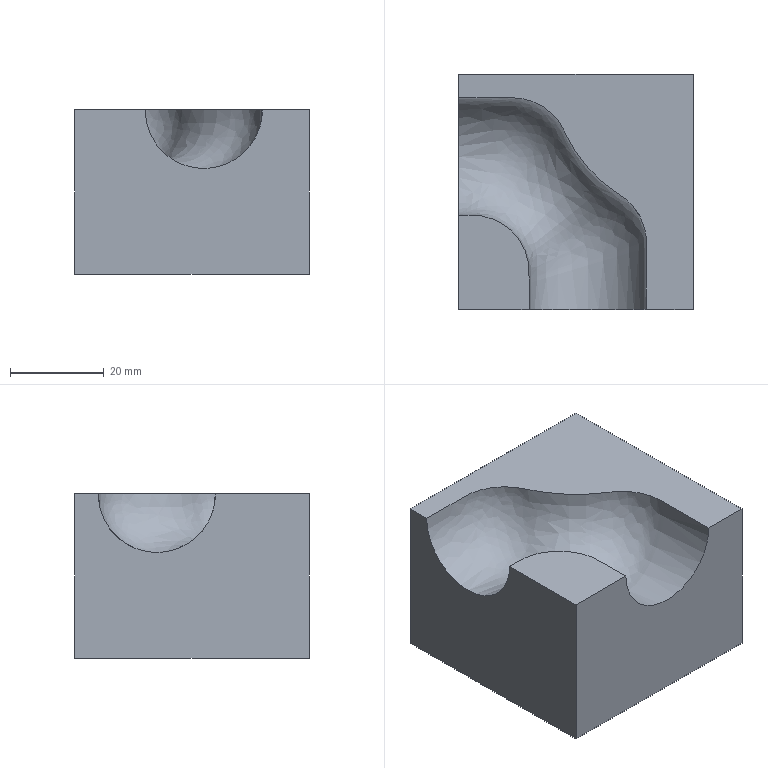NC program | NX | posted with a generic post | part box 50 x 50 x 35 mm
Lines 1308 to 2416 of 32931:
(CAVITY_MILL_COPY , TOOL : D6)
N2614 M6
N2616 G54
N2618 G17 G0 G90 X-3.401 Y23.101 S3000 M3
N2620 G43 Z10. H0
N2622 Z0.05
N2624 G94 G1 Z-0.15 F2500.
N2626 X0. Y23.1
N2628 X2.871 Y23.099
N2630 G2 X18.098 Y8.253 R15.092
N2632 G1 X18.102 Y0.
N2634 X18.103 Y-3.399
N2636 Z0.05
N2638 G0 Z0.3
N2640 X36.899
N2642 Z0.05
N2644 G1 Z-0.15
N2646 X36.898 Y0.
N2648 X36.896 Y14.233
N2650 G3 X32.772 Y21.732 R8.945
N2652 G2 X19.737 Y36.582 R33.162
N2654 G3 X11.611 Y41.89 R8.932
N2656 G1 X10.047 Y41.897
N2658 X0.479 Y41.896
N2660 X0. Y41.898
N2662 X-3.411 Y41.91
N2664 Z0.05
N2666 G0 Z0.3
N2668 X-3.404 Y23.103
N2670 Z-0.1
N2672 G1 Z-0.3
N2674 X0. Y23.104
N2676 X2.871
N2678 G2 X18.102 Y8.253 R15.093
N2680 G1 X18.106 Y0.
N2682 X18.108 Y-3.398
N2684 Z-0.1
N2686 G0 Z0.15
N2688 X36.894
N2690 Z-0.1
N2692 G1 Z-0.3
N2694 Y0.
N2696 X36.893 Y14.233
N2698 G3 X32.772 Y21.728 R8.987
N2700 G2 X19.732 Y36.58 R33.175
N2702 G3 X11.629 Y41.882 R8.925
N2704 G1 X10.047 Y41.891
N2706 X0.479 Y41.892
N2708 X0. Y41.894
N2710 X-3.413 Y41.906
N2712 Z-0.1
N2714 G0 Z0.15
N2716 X-3.408 Y23.105
N2718 Z-0.25
N2720 G1 Z-0.45
N2722 X0. Y23.108
N2724 X2.871 Y23.11
N2726 G2 X18.108 Y8.253 R15.1
N2728 G1 X18.111 Y0.
N2730 X18.113 Y-3.398
N2732 Z-0.25
N2734 G0 Z0.
N2736 X36.89 Y-3.4
N2738 Z-0.25
N2740 G1 Z-0.45
N2742 X36.889 Y0.
N2744 X36.888 Y14.233
N2746 G3 X32.772 Y21.72 R9.003
N2748 G2 X19.728 Y36.575 R33.21
N2750 G3 X11.589 Y41.872 R8.923
N2752 G1 X0. Y41.89
N2754 X-3.407 Y41.895
N2756 Z-0.25
N2758 G0 Z0.
N2760 X-3.414 Y23.106
N2762 Z-0.4
N2764 G1 Z-0.6
N2766 X0. Y23.113
N2768 X2.273 Y23.119
N2770 X2.871 Y23.118
N2772 G2 X11.91 Y20.213 R15.186
N2774 G1 X12.439 Y19.807
N2776 X12.677 Y19.615
N2778 X13.037 Y19.305
N2780 X13.386 Y19.017
N2782 G2 X17.883 Y10.645 R15.216
N2784 G1 X17.969 Y10.047
N2786 G2 X18.116 Y7.655 R16.334
N2788 G1 Y0.
N2790 Y-3.402
N2792 Z-0.4
N2794 G0 Z-0.15
N2796 X36.886 Y-3.405
N2798 Z-0.4
N2800 G1 Z-0.6
N2802 X36.885 Y0.
N2804 X36.883 Y14.233
N2806 G3 X32.772 Y21.713 R9.021
N2808 G2 X19.725 Y36.568 R33.239
N2810 G3 X11.607 Y41.864 R8.924
N2812 G1 X10.645 Y41.868
N2814 X0. Y41.879
N2816 X-3.4 Y41.882
N2818 Z-0.4
N2820 G0 Z-0.15
N2822 X-3.41 Y23.119
N2824 Z-0.55
N2826 G1 Z-0.75
N2828 X0. Y23.123
N2830 X2.871 Y23.125
N2832 G2 X11.841 Y20.272 R15.186
N2834 G1 X12.439 Y19.82
N2836 G2 X16.027 Y15.696 R14.321
N2838 X18.119 Y8.253 R15.038
N2840 G1 X18.124 Y0.
N2842 X18.126 Y-3.404
N2844 Z-0.55
N2846 G0 Z-0.3
N2848 X36.892 Y-3.42
N2850 Z-0.55
N2852 G1 Z-0.75
N2854 X36.875 Y0.
N2856 X36.873 Y0.479
N2858 X36.875 Y13.635
N2860 X36.871 Y14.233
N2862 G3 X32.772 Y21.699 R8.983
N2864 G2 X19.701 Y36.597 R33.251
N2866 G3 X11.648 Y41.855 R8.845
N2868 G1 X10.645 Y41.859
N2870 X0. Y41.867
N2872 X-3.398 Y41.87
N2874 Z-0.55
N2876 G0 Z-0.3
N2878 X-3.411 Y23.129
N2880 Z-0.7
N2882 G1 Z-0.9
N2884 X0. Y23.134
N2886 X2.871 Y23.138
N2888 X3.469 Y23.125
N2890 G2 X13.037 Y19.327 R15.12
N2892 G1 X13.42 Y19.017
N2894 G3 X14.233 Y18.183 R12.651
N2896 G1 X14.522 Y17.821
N2898 X14.831 Y17.439
N2900 X15.024 Y17.223
N2902 G2 X17.821 Y11.024 R15.031
N2904 G1 X17.903 Y10.645
N2906 X17.994 Y10.047
N2908 X18.066 Y9.449
N2910 X18.101 Y8.851
N2912 X18.131 Y8.253
N2914 X18.137 Y7.655
N2916 X18.144 Y0.479
N2918 X18.141 Y0.
N2920 X18.126 Y-3.415
N2922 Z-0.7
N2924 G0 Z-0.45
N2926 X36.877 Y-3.418
N2928 Z-0.7
N2930 G1 Z-0.9
N2932 X36.862 Y0.
N2934 X36.86 Y0.479
N2936 X36.863 Y13.635
N2938 X36.858 Y14.233
N2940 G3 X32.772 Y21.68 R8.913
N2942 G2 X21.689 Y32.772 R33.333
N2944 X19.726 Y36.529 R32.02
N2946 G3 X11.841 Y41.846 R8.916
N2948 G1 X0. Y41.856
N2950 X-3.398 Y41.859
N2952 Z-0.7
N2954 G0 Z-0.45
N2956 X-3.41 Y23.142
N2958 Z-0.85
N2960 G1 Z-1.05
N2962 X0. Y23.148
N2964 X2.871 Y23.154
N2966 X3.469 Y23.134
N2968 G2 X13.037 Y19.351 R15.19
N2970 G1 X13.437 Y19.017
N2972 X13.635 Y18.788
N2974 G2 X14.531 Y17.821 R7.059
N2976 X17.654 Y11.841 R14.809
N2978 X18.147 Y8.253 R15.68
N2980 G1 X18.153 Y7.655
N2982 X18.16 Y0.479
N2984 X18.158 Y0.
N2986 X18.144 Y-3.41
N2988 Z-0.85
N2990 G0 Z-0.6
N2992 X36.862 Y-3.417
N2994 Z-0.85
N2996 G1 Z-1.05
N2998 X36.848 Y0.
N3000 X36.846 Y0.479
N3002 X36.85 Y13.635
N3004 X36.846 Y14.233
N3006 G3 X33.37 Y21.256 R8.93
N3008 G1 X33.153 Y21.409
N3010 X32.257 Y22.007
N3012 X32.174 Y22.051
N3014 G2 X23.728 Y29.782 R32.398
N3016 X19.798 Y36.36 R32.22
N3018 G3 X17.757 Y39.35 R9.751
N3020 X11.841 Y41.837 R8.944
N3022 G1 X0. Y41.845
N3024 X-3.398 Y41.847
N3026 Z-0.85
N3028 G0 Z-0.6
N3030 X-3.411 Y23.156
N3032 Z-1.
N3034 G1 Z-1.2
N3036 X0. Y23.163
N3038 X2.871 Y23.169
N3040 X3.469 Y23.15
N3042 G2 X12.439 Y19.876 R15.361
N3044 X18.091 Y9.449 R15.063
N3046 G1 X18.163 Y8.253
N3048 X18.168 Y7.655
N3050 X18.175 Y0.
N3052 X18.177 Y-3.391
N3054 Z-1.
N3056 G0 Z-0.75
N3058 X36.847 Y-3.417
N3060 Z-1.
N3062 G1 Z-1.2
N3064 X36.835 Y0.
N3066 X36.833 Y0.479
N3068 X36.838 Y13.635
N3070 X36.834 Y14.271
N3072 G3 X33.321 Y21.261 R8.822
N3074 X32.174 Y22.034 R13.031
N3076 G2 X19.781 Y36.36 R32.749
N3078 G3 X17.746 Y39.35 R9.753
N3080 X11.841 Y41.829 R9.09
N3082 G1 X0. Y41.834
N3084 X-3.398 Y41.835
N3086 Z-1.
N3088 G0 Z-0.75
N3090 X-3.467 Y23.108
N3092 Z-1.15
N3094 G1 Z-1.35
N3096 X0. Y23.18
N3098 G2 X3.621 Y23.151 R62.449
N3100 X18.01 Y10.234 R15.109
N3102 X18.184 Y7.655 R16.706
N3104 G1 X18.192 Y0.008
N3106 Y0.
N3108 X18.187 Y-3.401
N3110 Z-1.15
N3112 G0 Z-0.9
N3114 X36.822 Y-3.407
N3116 Z-1.15
N3118 G1 Z-1.35
N3120 Y0.
N3122 X36.821 Y14.233
N3124 G3 X33.37 Y21.209 R8.848
N3126 G1 X33.095 Y21.409
N3128 X31.576 Y22.4
N3130 G2 X19.615 Y36.685 R32.788
N3132 G3 X13.635 Y41.577 R8.913
N3134 X11.841 Y41.82 R12.805
N3136 G1 X10.645 Y41.823
N3138 X0.479 Y41.821
N3140 X0. Y41.822
N3142 X-3.409 Y41.832
N3144 Z-1.15
N3146 G0 Z-0.9
N3148 X-3.415 Y23.184
N3150 Z-1.3
N3152 G1 Z-1.5
N3154 X0. Y23.193
N3156 X2.871 Y23.201
N3158 X3.469 Y23.183
N3160 G2 X17.347 Y13.037 R15.177
N3162 X18.195 Y8.253 R16.139
N3164 G1 X18.202 Y7.057
N3166 X18.209 Y0.007
N3168 Y0.
N3170 X18.205 Y-3.4
N3172 Z-1.3
N3174 G0 Z-1.05
N3176 X36.808 Y-3.41
N3178 Z-1.3
N3180 G1 Z-1.5
N3182 Y0.
N3184 X36.809 Y14.233
N3186 G3 X33.968 Y20.696 R8.958
N3188 X32.155 Y22.007 R14.236
N3190 G2 X19.743 Y36.36 R32.656
N3192 G3 X14.94 Y41.144 R8.948
N3194 X11.243 Y41.809 R9.702
N3196 G1 X0.479 Y41.804
N3198 X0. Y41.806
N3200 X-3.415 Y41.82
N3202 Z-1.3
N3204 G0 Z-1.05
N3206 X-3.422 Y23.197
N3208 Z-1.45
N3210 G1 Z-1.65
N3212 X0. Y23.211
N3214 X2.871 Y23.222
N3216 X3.469 Y23.199
N3218 G2 X17.369 Y13.037 R15.184
N3220 X18.212 Y7.93 R16.075
N3222 G1 X18.225 Y0.
N3224 X18.231 Y-3.39
N3226 Z-1.45
N3228 G0 Z-1.2
N3230 X36.784 Y-3.405
N3232 Z-1.45
N3234 G1 Z-1.65
N3236 Y0.
N3238 X36.788 Y14.233
N3240 G3 X33.37 Y21.161 R8.826
N3242 G1 X33.019 Y21.409
N3244 X31.208 Y22.605
N3246 G2 X19.721 Y36.36 R32.588
N3248 G3 X14.888 Y41.144 R8.922
N3250 X11.243 Y41.789 R9.65
N3252 G1 X0. Y41.786
N3254 X-3.403
N3256 Z-1.45
N3258 G0 Z-1.2
N3260 X-3.414 Y23.226
N3262 Z-1.6
N3264 G1 Z-1.8
N3266 X0. Y23.236
N3268 X2.871 Y23.245
N3270 X3.469 Y23.222
N3272 G2 X15.976 Y16.027 R15.288
N3274 X18.227 Y8.253 R15.352
N3276 G1 X18.231 Y7.655
N3278 X18.244 Y0.479
N3280 X18.243 Y0.
N3282 X18.237 Y-3.405
N3284 Z-1.6
N3286 G0 Z-1.35
N3288 X36.759 Y-3.4
N3290 Z-1.6
N3292 G1 Z-1.8
N3294 X36.76 Y0.
N3296 X36.766 Y14.233
N3298 G3 X32.772 Y21.561 R8.792
N3300 G2 X21.206 Y33.379 R32.856
N3302 X19.665 Y36.441 R31.796
N3304 G3 X11.841 Y41.767 R8.898
N3306 G1 X0. Y41.766
N3308 X-3.404
N3310 Z-1.6
N3312 G0 Z-1.35
N3314 X-3.405 Y23.254
N3316 Z-1.75
N3318 G1 Z-1.95
N3320 X0. Y23.262
N3322 X2.871 Y23.268
N3324 X3.469 Y23.247
N3326 G2 X14.233 Y18.363 R15.434
N3328 X18.243 Y8.253 R15.114
N3330 G1 X18.259 Y0.
N3332 X18.266 Y-3.399
N3334 Z-1.75
N3336 G0 Z-1.5
N3338 X36.734 Y-3.396
N3340 Z-1.75
N3342 G1 Z-1.95
N3344 X36.736 Y0.
N3346 X36.743 Y14.194
N3348 G3 X32.591 Y21.644 R8.751
N3350 G2 X26.792 Y26.126 R35.109
N3352 X19.641 Y36.444 R32.684
N3354 G3 X11.522 Y41.75 R8.859
N3356 G1 X0. Y41.745
N3358 X-3.406 Y41.744
N3360 Z-1.75
N3362 G0 Z-1.5
N3364 X-3.402 Y23.283
N3366 Z-1.9
N3368 G1 Z-2.1
N3370 X0. Y23.287
N3372 X2.871 Y23.291
N3374 X3.469 Y23.272
N3376 G2 X13.618 Y19.017 R15.495
N3378 X18.121 Y10.047 R14.77
N3380 X18.259 Y8.253 R12.285
N3382 G1 X18.281 Y0.
N3384 X18.29 Y-3.398
N3386 Z-1.9
N3388 G0 Z-1.65
N3390 X36.722 Y-3.407
N3392 Z-1.9
N3394 G1 Z-2.1
N3396 X36.712 Y0.
N3398 X36.71 Y0.479
N3400 X36.726 Y13.635
N3402 X36.721 Y14.233
N3404 G3 X32.772 Y21.504 R8.721
N3406 G2 X29.184 Y23.999 R38.773
N3408 X19.935 Y35.762 R32.106
N3410 G3 X19.262 Y37.142 R17.898
N3412 X11.562 Y41.724 R8.749
N3414 G1 X0. Y41.715
N3416 X-3.399 Y41.712
N3418 Z-1.9
N3420 G0 Z-1.65
N3422 X-3.401 Y23.312
N3424 Z-2.05
N3426 G1 Z-2.25
N3428 X0. Y23.313
N3430 X2.871 Y23.314
N3432 G2 X13.635 Y19.041 R15.623
N3434 X17.948 Y11.243 R14.636
N3436 X18.279 Y8.253 R14.6
N3438 G1 X18.311 Y0.
N3440 X18.324 Y-3.389
N3442 Z-2.05
N3444 G0 Z-1.8
N3446 X36.697 Y-3.408
N3448 Z-2.05
N3450 G1 Z-2.25
N3452 X36.687 Y0.
N3454 X36.686 Y0.479
N3456 X36.703 Y13.635
N3458 X36.699 Y14.233
N3460 G3 X32.772 Y21.474 R8.709
N3462 G2 X31.456 Y22.325 R116.378
N3464 X19.621 Y36.39 R32.097
N3466 G3 X11.535 Y41.692 R8.805
N3468 G1 X0. Y41.682
N3470 X-3.391 Y41.678
N3472 Z-2.05
N3474 G0 Z-1.8
N3476 X-3.404 Y23.341
N3478 Z-2.2
N3480 G1 Z-2.4
N3482 X0. Y23.338
N3484 X2.871 Y23.336
N3486 G2 X14.177 Y18.55 R15.647
N3488 X17.411 Y13.306 R14.466
N3490 X18.306 Y8.253 R15.847
N3492 G1 X18.341 Y0.005
N3494 Y0.
N3496 X18.349 Y-3.395
N3498 Z-2.2
N3500 G0 Z-1.95
N3502 X36.671 Y-3.41
N3504 Z-2.2
N3506 G1 Z-2.4
N3508 X36.663 Y0.
N3510 X36.662 Y0.479
N3512 X36.681 Y13.635
N3514 X36.677 Y14.233
N3516 G3 X32.772 Y21.445 R8.766
N3518 G2 X30.958 Y22.625 R53.384
N3520 X19.617 Y36.348 R31.874
N3522 G3 X11.528 Y41.661 R8.801
N3524 G1 X0.012 Y41.649
N3526 X0.
N3528 X-3.402 Y41.658
N3530 Z-2.2
N3532 G0 Z-1.95
N3534 X-3.39 Y23.39
N3536 Z-2.35
N3538 G1 Z-2.55
N3540 X0. Y23.367
N3542 X4.067 Y23.34
N3544 G2 X9.449 Y21.944 R16.364
N3546 X16.625 Y15.212 R15.269
N3548 X18.334 Y8.253 R15.742
N3550 G1 X18.371 Y0.007
N3552 Y0.
N3554 X18.379 Y-3.395
N3556 Z-2.35
N3558 G0 Z-2.1
N3560 X36.623 Y-3.393
N3562 Z-2.35
N3564 G1 Z-2.55
N3566 X36.629 Y0.
N3568 X36.652 Y14.233
N3570 G3 X33.968 Y20.455 R8.879
N3572 X32.174 Y21.802 R11.572
N3574 G1 X31.838 Y22.007
N3576 G2 X19.577 Y36.36 R31.869
N3578 G3 X11.841 Y41.625 R8.743
N3580 G1 X11.243 Y41.629
N3582 X0. Y41.615
N3584 X-3.374 Y41.611
N3586 Z-2.35
N3588 G0 Z-2.1
N3590 X-3.414 Y23.397
N3592 Z-2.5
N3594 G1 Z-2.7
N3596 X0. Y23.403
N3598 X0.479 Y23.404
N3600 X2.871 Y23.397
N3602 G2 X11.243 Y21.006 R15.591
N3604 G1 X11.559 Y20.811
N3606 G2 X17.585 Y13.037 R14.848
N3608 G1 X17.746 Y12.439
N3610 X17.821 Y12.176
N3612 X17.92 Y11.841
N3614 X18.085 Y11.001
N3616 G2 X18.362 Y8.213 R14.88
N3618 G1 X18.401 Y0.005
N3620 Y0.
N3622 X18.411 Y-3.394
N3624 Z-2.5
N3626 G0 Z-2.25
N3628 X36.595 Y-3.4
N3630 Z-2.5
N3632 G1 Z-2.7
N3634 X36.591 Y0.
N3636 Y0.009
N3638 X36.617 Y14.233
N3640 G3 X32.721 Y21.409 R8.731
N3642 G2 X30.287 Y23.01 R37.222
N3644 X19.546 Y36.349 R31.859
N3646 G3 X11.591 Y41.597 R8.672
N3648 X0. Y41.583 R2175.918
N3650 G1 X-3.382 Y41.569
N3652 Z-2.5
N3654 G0 Z-2.25
N3656 X-3.39 Y23.458
N3658 Z-2.65
N3660 G1 Z-2.85
N3662 X0. Y23.437
N3664 X3.469 Y23.416
N3666 X4.067 Y23.404
N3668 G2 X13.037 Y19.765 R16.14
N3670 X17.401 Y13.635 R14.643
N3672 X18.389 Y8.253 R15.767
N3674 G1 X18.437 Y0.479
N3676 X18.436 Y0.
N3678 X18.433 Y-3.401
N3680 Z-2.65
N3682 G0 Z-2.4
N3684 X36.56
N3686 Z-2.65
N3688 G1 Z-2.85
N3690 X36.553 Y0.
N3692 Y0.012
N3694 X36.581 Y14.145
N3696 G3 X32.453 Y21.535 R8.649
N3698 G2 X30.384 Y22.898 R38.101
N3700 X19.518 Y36.33 R31.759
N3702 G3 X11.588 Y41.566 R8.636
N3704 X0. Y41.55 R2397.27
N3706 G1 X-3.384 Y41.537
N3708 Z-2.65
N3710 G0 Z-2.4
N3712 X-3.432 Y23.445
N3714 Z-2.8
N3716 G1 Z-3.
N3718 X0. Y23.474
N3720 G2 X4.067 Y23.435 R114.595
N3722 X13.635 Y19.296 R16.118
N3724 X17.223 Y14.176 R14.563
N3726 X18.103 Y11.243 R13.453
N3728 X18.399 Y8.851 R12.147
N3730 G1 X18.417 Y8.253
N3732 X18.477 Y0.024
N3734 Y0.
N3736 X18.476 Y-3.399
N3738 Z-2.8
N3740 G0 Z-2.55
N3742 X36.525
N3744 Z-2.8
N3746 G1 Z-3.
N3748 X36.515 Y0.
N3750 X36.514 Y0.479
N3752 X36.545 Y14.141
N3754 G3 X32.378 Y21.54 R8.619
N3756 G2 X26.194 Y26.362 R32.949
N3758 X19.485 Y36.324 R32.257
N3760 G3 X11.563 Y41.535 R8.605
N3762 G1 X0. Y41.516
N3764 X-3.381 Y41.511
N3766 Z-2.8
N3768 G0 Z-2.55
N3770 X-3.412 Y23.504
N3772 Z-2.95
N3774 G1 Z-3.15
N3776 X0. Y23.509
N3778 X0.479 Y23.51
N3780 X2.871 Y23.501
N3782 G2 X15.429 Y17.399 R15.884
N3784 X18.419 Y9.019 R15.08
N3786 G1 X18.455 Y8.253
N3788 X18.518 Y0.03
N3790 X18.519 Y0.
N3792 X18.511 Y-3.401
N3794 Z-2.95
N3796 G0 Z-2.7
N3798 X36.487 Y-3.4
N3800 Z-2.95
N3802 G1 Z-3.15
N3804 X36.478 Y0.
N3806 X36.476 Y0.479
N3808 X36.509 Y14.17
N3810 G3 X32.348 Y21.52 R8.536
N3812 G2 X23.801 Y28.973 R31.85
N3814 X19.458 Y36.302 R33.633
N3816 G3 X11.528 Y41.504 R8.622
N3818 G1 X0. Y41.483
N3820 X-3.394 Y41.477
N3822 Z-2.95
N3824 G0 Z-2.7
N3826 X-3.388 Y23.565
N3828 Z-3.099
N3830 G1 Z-3.299
N3832 X0. Y23.554
N3834 X2.871 Y23.545
N3836 X3.469 Y23.527
N3838 G2 X15.429 Y17.481 R15.912
N3840 X18.473 Y8.851 R15.304
N3842 G1 X18.495 Y8.253
N3844 X18.561 Y0.479
N3846 Y0.008
N3848 Y0.
N3850 X18.551 Y-3.403
N3852 Z-3.099
N3854 G0 Z-2.85
N3856 X36.448 Y-3.402
N3858 Z-3.099
N3860 G1 Z-3.299
N3862 X36.44 Y0.
N3864 X36.439 Y0.479
N3866 X36.473 Y14.233
N3868 G3 X32.174 Y21.587 R8.587
N3870 G2 X19.615 Y35.882 R31.002
N3872 G1 X19.398 Y36.36
N3874 G3 X14.831 Y40.825 R8.68
N3876 X11.243 Y41.472 R9.147
N3878 G1 X0. Y41.45
N3880 X-3.399 Y41.444
N3882 Z-3.099
N3884 G0 Z-2.85
N3886 X-3.395 Y23.596
N3888 Z-3.249
N3890 G1 Z-3.449
N3892 X0. Y23.6
N3894 X0.479 Y23.601
N3896 X2.871 Y23.59
N3898 G2 X14.123 Y19.017 R16.236
N3900 X18.102 Y11.841 R14.382
N3902 X18.535 Y8.253 R17.344
N3904 G1 X18.603 Y0.479
N3906 Y0.006
N3908 Y0.
N3910 X18.596 Y-3.401
N3912 Z-3.249
N3914 G0 Z-2.999
N3916 X36.393 Y-3.389
N3918 Z-3.249
N3920 G1 Z-3.449
N3922 X36.403 Y0.
N3924 X36.444 Y14.097
N3926 G3 X32.219 Y21.513 R8.577
N3928 G2 X19.876 Y35.231 R30.645
N3930 G3 X19.017 Y37.047 R67.322
N3932 X11.243 Y41.439 R8.648
N3934 G1 X0. Y41.405
N3936 X-3.391 Y41.395
N3938 Z-3.249
N3940 G0 Z-2.999
N3942 X-3.395 Y23.642
N3944 Z-3.399
N3946 G1 Z-3.599
N3948 X0. Y23.645
N3950 X0.479 Y23.646
N3952 X2.871 Y23.635
N3954 G2 X12.827 Y20.213 R16.447
N3956 X18.273 Y11.243 R14.503
N3958 X18.574 Y8.253 R18.487
N3960 X18.644 Y0. R552.236
N3962 G1 X18.648 Y-3.39
N3964 Z-3.399
N3966 G0 Z-3.149
N3968 X36.356 Y-3.394
N3970 Z-3.399
N3972 G1 Z-3.599
N3974 X36.365 Y0.
N3976 X36.402 Y14.233
N3978 G3 X32.313 Y21.409 R8.54
N3980 G2 X19.593 Y35.762 R30.544
N3982 G1 X19.326 Y36.36
N3984 G3 X14.831 Y40.728 R8.668
N3986 X11.532 Y41.394 R8.382
N3988 G1 X0.01 Y41.357
N3990 X0.
N3992 X-3.399 Y41.358
N3994 Z-3.399
N3996 G0 Z-3.149
N3998 X-3.382 Y23.702
N4000 Z-3.549
N4002 G1 Z-3.749
N4004 X0. Y23.69
N4006 X2.871 Y23.68
N4008 G2 X12.907 Y20.213 R16.586
N4010 X18.311 Y11.273 R14.449
N4012 X18.605 Y8.117 R19.633
N4014 G1 X18.684 Y1.675
N4016 X18.686 Y0.
N4018 X18.69 Y-3.394
N4020 Z-3.549
N4022 G0 Z-3.299
N4024 X36.309 Y-3.396
N4026 Z-3.549
N4028 G1 Z-3.749
N4030 X36.315 Y0.
N4032 Y0.007
N4034 X36.372 Y14.061
N4036 G3 X32.147 Y21.459 R8.529
N4038 G2 X19.431 Y36.032 R30.345
N4040 G3 X11.444 Y41.347 R8.616
N4042 G1 X0.012 Y41.309
N4044 X0.
N4046 X-3.399 Y41.311
N4048 Z-3.549
N4050 G0 Z-3.299
N4052 X-3.366 Y23.761
N4054 Z-3.699
N4056 G1 Z-3.899
N4058 X0. Y23.735
N4060 X3.469 Y23.708
N4062 X4.067 Y23.684
N4064 G2 X13.737 Y19.615 R17.005
N4066 X18.245 Y11.841 R14.598
N4068 G1 X18.357 Y11.26
N4070 G2 X18.643 Y8.452 R15.877
N4072 G1 X18.728 Y1.675
N4074 X18.731 Y0.
N4076 X18.736 Y-3.395
N4078 Z-3.699
N4080 G0 Z-3.449
N4082 X36.248 Y-3.378
N4084 Z-3.699
N4086 G1 Z-3.899
N4088 X36.263 Y0.
N4090 X36.327 Y14.044
N4092 G3 X32.113 Y21.429 R8.509
N4094 G2 X26.519 Y25.596 R31.428
N4096 G3 X25.596 Y26.511 R11.013
N4098 G2 X22.858 Y29.782 R39.083
N4100 X19.321 Y36.14 R34.678
N4102 G3 X11.483 Y41.301 R8.487
N4104 G1 X0.012 Y41.261
N4106 X0.
N4108 X-3.399 Y41.263
N4110 Z-3.699
N4112 G0 Z-3.449
N4114 X-3.364 Y23.806
N4116 Z-3.849
N4118 G1 Z-4.049
N4120 X0. Y23.78
N4122 X3.469 Y23.753
N4124 X4.067 Y23.731
N4126 G2 X13.827 Y19.615 R17.115
N4128 X17.326 Y14.831 R15.134
N4130 X18.679 Y8.851 R16.835
N4132 G1 X18.693 Y8.253
N4134 X18.786 Y0.479
N4136 Y0.005
N4138 Y0.
N4140 X18.783 Y-3.4
N4142 Z-3.849
N4144 G0 Z-3.599
N4146 X36.195 Y-3.375
N4148 Z-3.849
N4150 G1 Z-4.049
N4152 X36.211 Y0.
N4154 X36.277 Y14.054
N4156 G3 X32.06 Y21.396 R8.431
N4158 G2 X27.12 Y24.998 R28.735
N4160 X26.194 Y25.863 R5.21
N4162 X24.727 Y27.39 R15.376
N4164 X20.914 Y32.772 R28.878
N4166 X19.251 Y36.187 R42.129
N4168 G3 X11.509 Y41.256 R8.401
N4170 G1 X0.009 Y41.213
N4172 X0.
N4174 X-3.397 Y41.21
N4176 Z-3.849
N4178 G0 Z-3.599
N4180 X-3.405 Y23.809
N4182 Z-3.999
N4184 G1 Z-4.199
N4186 X0. Y23.835
N4188 G2 X4.067 Y23.777 R94.103
N4190 X13.917 Y19.615 R17.183
N4192 G1 X14.413 Y19.125
N4194 G2 X18.419 Y11.421 R14.174
N4196 X18.721 Y8.851 R15.586
N4198 G1 X18.836 Y1.675
N4200 X18.841 Y0.015
N4202 Y0.
N4204 X18.834 Y-3.401
N4206 Z-3.999
N4208 G0 Z-3.749
N4210 X36.166 Y-3.396
N4212 Z-3.999
N4214 G1 Z-4.199
N4216 X36.158 Y0.
N4218 X36.157 Y0.479
N4220 X36.228 Y14.068
N4222 G3 X32.046 Y21.342 R8.341
N4224 G2 X20.213 Y34.004 R29.586
N4226 X19.126 Y36.36 R68.823
N4228 G3 X11.243 Y41.208 R8.419
N4230 G1 X0. Y41.165
N4232 X-3.386 Y41.153
N4234 Z-3.999
N4236 G0 Z-3.749
N4238 X-3.359 Y23.926
N4240 Z-4.149
N4242 G1 Z-4.349
N4244 X0. Y23.892
N4246 X3.469 Y23.856
N4248 X4.067 Y23.83
N4250 G2 X13.037 Y20.408 R17.327
N4252 X17.467 Y14.831 R14.499
N4254 X18.779 Y8.484 R17.39
N4256 G1 X18.891 Y1.675
N4258 X18.896 Y0.018
N4260 Y0.
N4262 X18.889 Y-3.402
N4264 Z-4.149
N4266 G0 Z-3.899
N4268 X36.113 Y-3.398
N4270 Z-4.149
N4272 G1 Z-4.349
N4274 X36.106 Y0.
N4276 X36.105 Y0.479
N4278 X36.178 Y14.047
N4280 G3 X32.113 Y21.243 R8.322
N4282 G1 X31.576 Y21.563
N4284 G2 X20.479 Y33.37 R29.133
N4286 X19.178 Y36.123 R52.03
N4288 G3 X11.435 Y41.163 R8.409
N4290 G1 X0. Y41.111
N4292 X-3.381 Y41.095
N4294 Z-4.149
N4296 G0 Z-3.899
N4298 X-3.367 Y23.985
N4300 Z-4.299
N4302 G1 Z-4.499
N4304 X0. Y23.951
N4306 X3.469 Y23.915
N4308 X4.067 Y23.89
N4310 G2 X14.097 Y19.615 R17.419
N4312 X18.321 Y12.439 R14.096
N4314 G1 X18.419 Y11.977
N4316 G2 X18.839 Y8.253 R18.33
N4318 X18.952 Y0.017 R443.026
N4320 G1 Y0.
N4322 X18.948 Y-3.4
N4324 Z-4.299
N4326 G0 Z-4.049
N4328 X36.061 Y-3.403
N4330 Z-4.299
N4332 G1 Z-4.499
N4334 X36.052 Y0.
N4336 X36.051 Y0.479
N4338 X36.129 Y14.041
N4340 G3 X31.972 Y21.259 R8.263
N4342 G2 X23.458 Y28.586 R29.649
N4344 X19.301 Y35.762 R30.534
N4346 G3 X11.243 Y41.109 R8.435
N4348 G2 X0. Y41.049 R909.556
N4350 G1 X-3.39 Y41.052
N4352 Z-4.299
N4354 G0 Z-4.049
N4356 X-3.368 Y24.044
N4358 Z-4.449
N4360 G1 Z-4.649
N4362 X0. Y24.01
N4364 X3.469 Y23.974
N4366 X4.067 Y23.949
N4368 G2 X13.635 Y20.104 R17.76
N4370 X18.379 Y12.439 R14.028
N4372 X18.89 Y8.253 R18.463
N4374 X19.007 Y0. R440.117
N4376 G1 X19.023 Y-3.38
N4378 Z-4.449
N4380 G0 Z-4.199
N4382 X36.001 Y-3.403
N4384 Z-4.449
N4386 G1 Z-4.649
N4388 X35.99 Y0.
N4390 X35.989 Y0.011
N4392 G2 X36.081 Y13.952 R1128.596
N4394 G3 X31.937 Y21.212 R8.248
N4396 G2 X25.447 Y26.194 R30.61
N4398 X19.241 Y35.762 R30.012
N4400 G3 X11.243 Y41.051 R8.396
N4402 G2 X0. Y40.989 R847.691
N4404 G1 X-3.401 Y40.992
N4406 Z-4.449
N4408 G0 Z-4.199
N4410 X-3.369 Y24.104
N4412 Z-4.599
N4414 G1 Z-4.799
N4416 X0. Y24.069
N4418 X3.469 Y24.033
N4420 X4.067 Y24.009
N4422 G2 X13.635 Y20.183 R17.802
N4424 X18.443 Y12.439 R13.903
N4426 X18.941 Y8.253 R18.699
N4428 G1 X18.95 Y7.655
N4430 G2 X19.075 Y0. R394.9
N4432 G1 X19.097 Y-3.365
N4434 Z-4.599
N4436 G0 Z-4.349
N4438 X35.94 Y-3.404
N4440 Z-4.599
N4442 G1 Z-4.799
N4444 X35.926 Y0.
N4446 Y0.013
N4448 G2 X36.021 Y13.635 R1009.341
N4450 G1 X36.012 Y14.233
N4452 G3 X32.174 Y21.003 R8.18
N4454 G2 X26.194 Y25.356 R32.536
N4456 X19.181 Y35.762 R29.502
N4458 G3 X15.429 Y39.999 R8.576
N4460 X11.243 Y40.993 R8.403
N4462 G2 X0. Y40.928 R807.245
N4464 G1 X-3.401 Y40.932
N4466 Z-4.599
N4468 G0 Z-4.349
N4470 X-3.348 Y24.172
N4472 Z-4.749
N4474 G1 Z-4.949
N4476 X0. Y24.133
N4478 X3.469 Y24.092
N4480 X4.067 Y24.068
N4482 G2 X9.753 Y22.605 R17.343
N4484 X14.831 Y19.213 R16.701
N4486 X17.495 Y15.429 R15.097
N4488 X18.949 Y9.449 R17.064
N4490 G1 X18.983 Y8.851
N4492 X19.136 Y1.675
N4494 X19.146 Y0.
N4496 X19.166 Y-3.357
N4498 Z-4.749
N4500 G0 Z-4.499
N4502 X35.874 Y-3.403
N4504 Z-4.749
N4506 G1 Z-4.949
N4508 X35.863 Y0.
N4510 Y0.016
N4512 G2 X35.952 Y14.233 R1693.507
N4514 G3 X32.174 Y20.929 R8.126
N4516 G2 X26.194 Y25.249 R32.384
N4518 X19.121 Y35.762 R29.376
N4520 G3 X11.243 Y40.934 R8.269
N4522 G2 X0. Y40.867 R658.067
N4524 G1 X-3.409 Y40.876
N4526 Z-4.749
N4528 G0 Z-4.499
N4530 X-3.402 Y24.195
N4532 Z-4.899
N4534 G1 Z-5.099
N4536 X0. Y24.203
N4538 X0.03
N4540 X2.871 Y24.181
N4542 X3.469 Y24.16
N4544 G2 X8.253 Y23.252 R15.966
N4546 X13.84 Y20.213 R17.998
N4548 X18.258 Y13.635 R13.797
N4550 X19.005 Y9.449 R17.517
N4552 X19.217 Y0.035 R289.341
N4554 G1 Y0.
N4556 X19.199 Y-3.393
N4558 Z-4.899
N4560 G0 Z-4.649
N4562 X35.792 Y-3.384
N4564 Z-4.899
N4566 G1 Z-5.099
N4568 X35.8 Y0.
N4570 G2 X35.889 Y13.983 R1832.524
N4572 G3 X31.755 Y21.109 R8.067
N4574 G2 X24.036 Y27.39 R28.748
N4576 X19.017 Y35.856 R30.434
N4578 G3 X11.243 Y40.876 R8.257
N4580 G2 X0. Y40.8 R588.962
N4582 G1 X-3.407 Y40.809
N4584 Z-4.899
N4586 G0 Z-4.649
N4588 X-3.369 Y24.298
N4590 Z-5.049
N4592 G1 Z-5.249
N4594 X0. Y24.272
N4596 X2.871 Y24.25
N4598 G2 X8.584 Y23.203 R16.565
N4600 X13.966 Y20.213 R18.14
N4602 X18.335 Y13.635 R13.774
N4604 X19.071 Y9.449 R18.207
N4606 X19.288 Y0.038 R270.629
N4608 G1 Y0.
N4610 X19.266 Y-3.396
N4612 Z-5.049
N4614 G0 Z-4.799
N4616 X35.756 Y-3.41
N4618 Z-5.049
N4620 G1 Z-5.249
N4622 X35.727 Y0.
N4624 Y0.03
N4626 G2 X35.841 Y13.635 R935.595
N4628 G3 X31.576 Y21.131 R8.115
N4630 G2 X24.453 Y26.792 R28.737
N4632 X19.017 Y35.715 R29.382
N4634 G3 X11.243 Y40.813 R8.216
N4636 G2 X0. Y40.729 R625.434
N4638 G1 X-3.38 Y40.733
N4640 Z-5.049
N4642 G0 Z-4.799
N4644 X-3.343 Y24.368
N4646 Z-5.199
N4648 G1 Z-5.399
N4650 X0. Y24.342
N4652 X2.871 Y24.319
N4654 X3.469 Y24.298
N4656 G2 X5.861 Y24.032 R14.447
N4658 X13.322 Y20.811 R19.238
N4660 X18.586 Y13.02 R13.688
N4662 X19.158 Y8.993 R19.888
N4664 X19.359 Y0. R274.505
N4666 G1 X19.379 Y-3.359
N4668 Z-5.199
N4670 G0 Z-4.949
N4672 X35.65 Y-3.373
N4674 Z-5.199
N4676 G1 Z-5.399
N4678 X35.652 Y0.
N4680 G2 X35.781 Y13.635 R781.256
N4682 G3 X31.576 Y21.052 R8.071
N4684 G2 X25.484 Y25.596 R29.44
N4686 X19.017 Y35.548 R28.527
N4688 G3 X16.007 Y39.35 R8.548
N4690 X11.243 Y40.745 R8.275
N4692 G2 X0. Y40.657 R641.261
N4694 G1 X-3.401 Y40.66
N4696 Z-5.199
N4698 G0 Z-4.949
N4700 X-3.403 Y24.402
N4702 Z-5.349
N4704 G1 Z-5.549
N4706 X0. Y24.413
N4708 X0.042
N4710 X2.871 Y24.388
N4712 X3.895 Y24.353
N4714 G2 X5.263 Y24.216 R10.33
N4716 X13.037 Y21.115 R19.827
N4718 X18.662 Y13.037 R13.697
N4720 X19.254 Y8.253 R21.399
N4722 G1 X19.268 Y7.655
N4724 X19.283 Y7.057
N4726 X19.324 Y5.861
N4728 G2 X19.431 Y0. R166.857
N4730 G1 X19.433 Y-3.377
N4732 Z-5.349
N4734 G0 Z-5.099
N4736 X35.574 Y-3.385
N4738 Z-5.349
N4740 G1 Z-5.549
N4742 X35.573 Y0.
N4744 Y0.002
N4746 G2 X35.711 Y13.635 R703.665
N4748 G3 X31.851 Y20.811 R7.995
N4750 G2 X24.998 Y25.953 R29.776
N4752 X19.017 Y35.381 R28.706
N4754 G3 X16.625 Y38.79 R8.723
N4756 X11.243 Y40.677 R8.134
N4758 G2 X0. Y40.586 R633.422
N4760 G1 X-3.402 Y40.588
N4762 Z-5.349
N4764 G0 Z-5.099
N4766 X-3.463 Y24.409
N4768 Z-5.499
N4770 G1 Z-5.699
N4772 X0. Y24.497
N4774 X0.1 Y24.498
N4776 X1.857 Y24.495
N4778 G2 X5.263 Y24.284 R28.536
N4780 X12.727 Y21.409 R19.715
N4782 G1 X12.767 Y21.385
N4784 G2 X18.791 Y12.82 R13.554
N4786 X19.322 Y8.253 R22.039
N4788 G1 X19.336 Y7.655
N4790 X19.352 Y7.057
N4792 X19.393 Y5.861
N4794 G2 X19.502 Y0. R167.552
N4796 G1 X19.505 Y-3.382
N4798 Z-5.499
N4800 G0 Z-5.249
N4802 X35.512 Y-3.393
N4804 Z-5.499
N4806 G1 Z-5.699
N4808 X35.495 Y0.
N4810 Y0.017
N4812 G2 X35.637 Y13.635 R684.581
N4814 G3 X31.576 Y20.895 R7.948
N4816 G2 X19.615 Y33.805 R26.889
N4818 X18.768 Y35.762 R136.94
N4820 G3 X11.243 Y40.609 R7.989
N4822 G2 X0. Y40.508 R659.544
N4824 G1 X-3.396 Y40.506